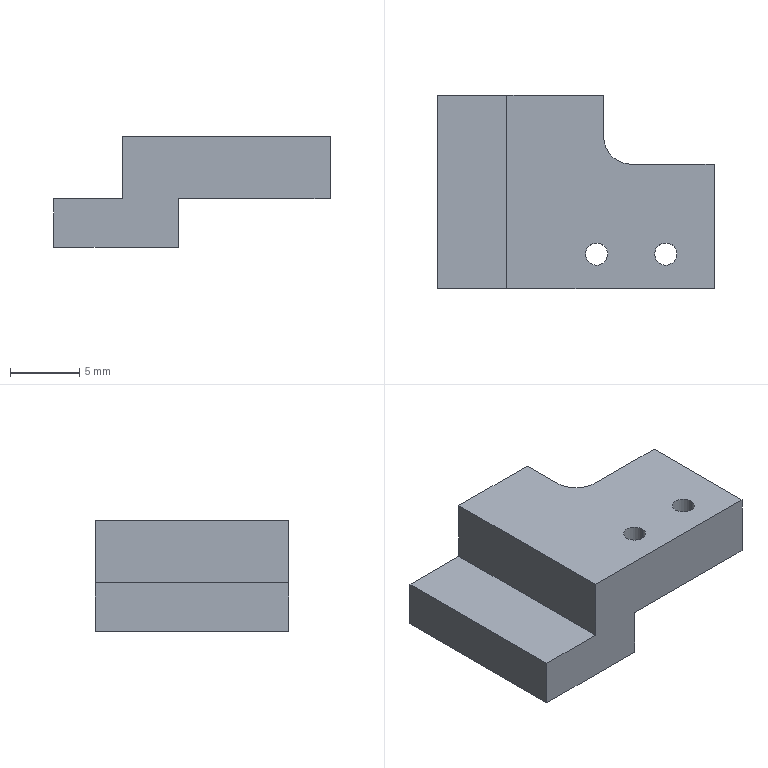Part | STEP file | FBDS-CS-024 | 1 solid | 19 faces | box 20 x 14 x 8 mm | volume 1034 mm3 | plane 14 | cylinder 5 | commonest cylinder face diameters 1.6 x4 4 x1
STEP:
#1=CARTESIAN_POINT('',(12.3,-11.5,5.));
#2=VERTEX_POINT('',#1);
#3=CARTESIAN_POINT('',(10.7,-11.5,5.));
#4=VERTEX_POINT('',#3);
#5=CARTESIAN_POINT('',(11.5,-11.5,5.));
#6=DIRECTION('',(0.,0.,-1.));
#7=DIRECTION('',(-1.,0.,0.));
#8=AXIS2_PLACEMENT_3D('',#5,#6,#7);
#9=CIRCLE('',#8,0.8);
#10=EDGE_CURVE('',#2,#4,#9,.T.);
#11=ORIENTED_EDGE('',*,*,#10,.T.);
#12=CARTESIAN_POINT('',(10.7,-11.5,8.));
#13=VERTEX_POINT('',#12);
#14=CARTESIAN_POINT('',(10.7,-11.5,8.));
#15=DIRECTION('',(0.,0.,1.));
#16=VECTOR('',#15,1000.);
#17=LINE('',#14,#16);
#18=EDGE_CURVE('',#4,#13,#17,.T.);
#19=ORIENTED_EDGE('',*,*,#18,.T.);
#20=CARTESIAN_POINT('',(12.3,-11.5,8.));
#21=VERTEX_POINT('',#20);
#22=CARTESIAN_POINT('',(11.5,-11.5,8.));
#23=DIRECTION('',(0.,0.,1.));
#24=DIRECTION('',(1.,0.,0.));
#25=AXIS2_PLACEMENT_3D('',#22,#23,#24);
#26=CIRCLE('',#25,0.8);
#27=EDGE_CURVE('',#13,#21,#26,.T.);
#28=ORIENTED_EDGE('',*,*,#27,.T.);
#29=CARTESIAN_POINT('',(12.3,-11.5,8.));
#30=DIRECTION('',(0.,0.,1.));
#31=VECTOR('',#30,1000.);
#32=LINE('',#29,#31);
#33=EDGE_CURVE('',#2,#21,#32,.T.);
#34=ORIENTED_EDGE('',*,*,#33,.F.);
#35=EDGE_LOOP('',(#11,#19,#28,#34));
#36=FACE_OUTER_BOUND('',#35,.T.);
#37=CARTESIAN_POINT('',(11.5,-11.5,8.));
#38=DIRECTION('',(0.,0.,1.));
#39=DIRECTION('',(1.,0.,0.));
#40=AXIS2_PLACEMENT_3D('',#37,#38,#39);
#41=CYLINDRICAL_SURFACE('',#40,0.8);
#42=ADVANCED_FACE('',(#36),#41,.F.);
#43=CARTESIAN_POINT('',(17.3,-11.5,5.));
#44=VERTEX_POINT('',#43);
#45=CARTESIAN_POINT('',(15.7,-11.5,5.));
#46=VERTEX_POINT('',#45);
#47=CARTESIAN_POINT('',(16.5,-11.5,5.));
#48=DIRECTION('',(0.,0.,-1.));
#49=DIRECTION('',(-1.,0.,0.));
#50=AXIS2_PLACEMENT_3D('',#47,#48,#49);
#51=CIRCLE('',#50,0.8);
#52=EDGE_CURVE('',#44,#46,#51,.T.);
#53=ORIENTED_EDGE('',*,*,#52,.T.);
#54=CARTESIAN_POINT('',(15.7,-11.5,8.));
#55=VERTEX_POINT('',#54);
#56=CARTESIAN_POINT('',(15.7,-11.5,8.));
#57=DIRECTION('',(0.,0.,1.));
#58=VECTOR('',#57,1000.);
#59=LINE('',#56,#58);
#60=EDGE_CURVE('',#46,#55,#59,.T.);
#61=ORIENTED_EDGE('',*,*,#60,.T.);
#62=CARTESIAN_POINT('',(17.3,-11.5,8.));
#63=VERTEX_POINT('',#62);
#64=CARTESIAN_POINT('',(16.5,-11.5,8.));
#65=DIRECTION('',(0.,0.,1.));
#66=DIRECTION('',(1.,0.,0.));
#67=AXIS2_PLACEMENT_3D('',#64,#65,#66);
#68=CIRCLE('',#67,0.8);
#69=EDGE_CURVE('',#55,#63,#68,.T.);
#70=ORIENTED_EDGE('',*,*,#69,.T.);
#71=CARTESIAN_POINT('',(17.3,-11.5,8.));
#72=DIRECTION('',(0.,0.,1.));
#73=VECTOR('',#72,1000.);
#74=LINE('',#71,#73);
#75=EDGE_CURVE('',#44,#63,#74,.T.);
#76=ORIENTED_EDGE('',*,*,#75,.F.);
#77=EDGE_LOOP('',(#53,#61,#70,#76));
#78=FACE_OUTER_BOUND('',#77,.T.);
#79=CARTESIAN_POINT('',(16.5,-11.5,8.));
#80=DIRECTION('',(0.,0.,1.));
#81=DIRECTION('',(1.,0.,0.));
#82=AXIS2_PLACEMENT_3D('',#79,#80,#81);
#83=CYLINDRICAL_SURFACE('',#82,0.8);
#84=ADVANCED_FACE('',(#78),#83,.F.);
#85=CARTESIAN_POINT('',(5.,-14.,3.5));
#86=VERTEX_POINT('',#85);
#87=CARTESIAN_POINT('',(0.,-14.,3.5));
#88=VERTEX_POINT('',#87);
#89=CARTESIAN_POINT('',(9.,-14.,3.5));
#90=DIRECTION('',(-1.,0.,0.));
#91=VECTOR('',#90,1000.);
#92=LINE('',#89,#91);
#93=EDGE_CURVE('',#86,#88,#92,.T.);
#94=ORIENTED_EDGE('',*,*,#93,.F.);
#95=CARTESIAN_POINT('',(5.,0.,3.5));
#96=VERTEX_POINT('',#95);
#97=CARTESIAN_POINT('',(5.,0.,3.5));
#98=DIRECTION('',(0.,1.,0.));
#99=VECTOR('',#98,1000.);
#100=LINE('',#97,#99);
#101=EDGE_CURVE('',#86,#96,#100,.T.);
#102=ORIENTED_EDGE('',*,*,#101,.T.);
#103=CARTESIAN_POINT('',(0.,0.,3.5));
#104=VERTEX_POINT('',#103);
#105=CARTESIAN_POINT('',(0.,0.,3.5));
#106=DIRECTION('',(-1.,0.,0.));
#107=VECTOR('',#106,1000.);
#108=LINE('',#105,#107);
#109=EDGE_CURVE('',#96,#104,#108,.T.);
#110=ORIENTED_EDGE('',*,*,#109,.T.);
#111=CARTESIAN_POINT('',(0.,0.,3.5));
#112=DIRECTION('',(0.,-1.,0.));
#113=VECTOR('',#112,1000.);
#114=LINE('',#111,#113);
#115=EDGE_CURVE('',#104,#88,#114,.T.);
#116=ORIENTED_EDGE('',*,*,#115,.T.);
#117=EDGE_LOOP('',(#94,#102,#110,#116));
#118=FACE_OUTER_BOUND('',#117,.T.);
#119=CARTESIAN_POINT('',(0.,0.,3.5));
#120=DIRECTION('',(0.,0.,1.));
#121=DIRECTION('',(1.,0.,0.));
#122=AXIS2_PLACEMENT_3D('',#119,#120,#121);
#123=PLANE('',#122);
#124=ADVANCED_FACE('',(#118),#123,.T.);
#125=CARTESIAN_POINT('',(9.,-14.,3.5));
#126=VERTEX_POINT('',#125);
#127=CARTESIAN_POINT('',(9.,-14.,0.));
#128=VERTEX_POINT('',#127);
#129=CARTESIAN_POINT('',(9.,-14.,8.64));
#130=DIRECTION('',(0.,0.,-1.));
#131=VECTOR('',#130,1000.);
#132=LINE('',#129,#131);
#133=EDGE_CURVE('',#126,#128,#132,.T.);
#134=ORIENTED_EDGE('',*,*,#133,.F.);
#135=CARTESIAN_POINT('',(20.,-14.,3.5));
#136=VERTEX_POINT('',#135);
#137=CARTESIAN_POINT('',(0.,-14.,3.5));
#138=DIRECTION('',(-1.,0.,0.));
#139=VECTOR('',#138,1000.);
#140=LINE('',#137,#139);
#141=EDGE_CURVE('',#136,#126,#140,.T.);
#142=ORIENTED_EDGE('',*,*,#141,.F.);
#143=CARTESIAN_POINT('',(20.,-14.,8.));
#144=VERTEX_POINT('',#143);
#145=CARTESIAN_POINT('',(20.,-14.,8.));
#146=DIRECTION('',(0.,0.,-1.));
#147=VECTOR('',#146,1000.);
#148=LINE('',#145,#147);
#149=EDGE_CURVE('',#144,#136,#148,.T.);
#150=ORIENTED_EDGE('',*,*,#149,.F.);
#151=CARTESIAN_POINT('',(5.,-14.,8.));
#152=VERTEX_POINT('',#151);
#153=CARTESIAN_POINT('',(0.,-14.,8.));
#154=DIRECTION('',(1.,0.,0.));
#155=VECTOR('',#154,1000.);
#156=LINE('',#153,#155);
#157=EDGE_CURVE('',#152,#144,#156,.T.);
#158=ORIENTED_EDGE('',*,*,#157,.F.);
#159=CARTESIAN_POINT('',(5.,-14.,-3.208));
#160=DIRECTION('',(0.,0.,1.));
#161=VECTOR('',#160,1000.);
#162=LINE('',#159,#161);
#163=EDGE_CURVE('',#86,#152,#162,.T.);
#164=ORIENTED_EDGE('',*,*,#163,.F.);
#165=ORIENTED_EDGE('',*,*,#93,.T.);
#166=CARTESIAN_POINT('',(0.,-14.,0.));
#167=VERTEX_POINT('',#166);
#168=CARTESIAN_POINT('',(0.,-14.,20.143));
#169=DIRECTION('',(0.,0.,-1.));
#170=VECTOR('',#169,1000.);
#171=LINE('',#168,#170);
#172=EDGE_CURVE('',#88,#167,#171,.T.);
#173=ORIENTED_EDGE('',*,*,#172,.T.);
#174=CARTESIAN_POINT('',(9.,-14.,0.));
#175=DIRECTION('',(-1.,0.,0.));
#176=VECTOR('',#175,1000.);
#177=LINE('',#174,#176);
#178=EDGE_CURVE('',#128,#167,#177,.T.);
#179=ORIENTED_EDGE('',*,*,#178,.F.);
#180=EDGE_LOOP('',(#134,#142,#150,#158,#164,#165,#173,#179));
#181=FACE_OUTER_BOUND('',#180,.T.);
#182=CARTESIAN_POINT('',(0.,-14.,8.));
#183=DIRECTION('',(0.,1.,0.));
#184=DIRECTION('',(0.,0.,1.));
#185=AXIS2_PLACEMENT_3D('',#182,#183,#184);
#186=PLANE('',#185);
#187=ADVANCED_FACE('',(#181),#186,.F.);
#188=CARTESIAN_POINT('',(20.,-13.5,3.5));
#189=VERTEX_POINT('',#188);
#190=CARTESIAN_POINT('',(20.,0.,3.5));
#191=DIRECTION('',(0.,-1.,0.));
#192=VECTOR('',#191,1000.);
#193=LINE('',#190,#192);
#194=EDGE_CURVE('',#189,#136,#193,.T.);
#195=ORIENTED_EDGE('',*,*,#194,.F.);
#196=CARTESIAN_POINT('',(20.,-13.5,5.));
#197=VERTEX_POINT('',#196);
#198=CARTESIAN_POINT('',(20.,-13.5,8.));
#199=DIRECTION('',(0.,0.,1.));
#200=VECTOR('',#199,1000.);
#201=LINE('',#198,#200);
#202=EDGE_CURVE('',#189,#197,#201,.T.);
#203=ORIENTED_EDGE('',*,*,#202,.T.);
#204=CARTESIAN_POINT('',(20.,-5.,5.));
#205=VERTEX_POINT('',#204);
#206=CARTESIAN_POINT('',(20.,0.,5.));
#207=DIRECTION('',(0.,-1.,0.));
#208=VECTOR('',#207,1000.);
#209=LINE('',#206,#208);
#210=EDGE_CURVE('',#205,#197,#209,.T.);
#211=ORIENTED_EDGE('',*,*,#210,.F.);
#212=CARTESIAN_POINT('',(20.,-5.,8.));
#213=VERTEX_POINT('',#212);
#214=CARTESIAN_POINT('',(20.,-5.,-2.5));
#215=DIRECTION('',(0.,0.,1.));
#216=VECTOR('',#215,1000.);
#217=LINE('',#214,#216);
#218=EDGE_CURVE('',#205,#213,#217,.T.);
#219=ORIENTED_EDGE('',*,*,#218,.T.);
#220=CARTESIAN_POINT('',(20.,0.,8.));
#221=DIRECTION('',(0.,1.,0.));
#222=VECTOR('',#221,1000.);
#223=LINE('',#220,#222);
#224=EDGE_CURVE('',#144,#213,#223,.T.);
#225=ORIENTED_EDGE('',*,*,#224,.F.);
#226=ORIENTED_EDGE('',*,*,#149,.T.);
#227=EDGE_LOOP('',(#195,#203,#211,#219,#225,#226));
#228=FACE_OUTER_BOUND('',#227,.T.);
#229=CARTESIAN_POINT('',(20.,0.,8.));
#230=DIRECTION('',(-1.,0.,0.));
#231=DIRECTION('',(0.,0.,1.));
#232=AXIS2_PLACEMENT_3D('',#229,#230,#231);
#233=PLANE('',#232);
#234=ADVANCED_FACE('',(#228),#233,.F.);
#235=CARTESIAN_POINT('',(9.,-13.5,3.5));
#236=VERTEX_POINT('',#235);
#237=CARTESIAN_POINT('',(28.367,-13.5,3.5));
#238=DIRECTION('',(1.,0.,0.));
#239=VECTOR('',#238,1000.);
#240=LINE('',#237,#239);
#241=EDGE_CURVE('',#236,#189,#240,.T.);
#242=ORIENTED_EDGE('',*,*,#241,.F.);
#243=CARTESIAN_POINT('',(9.,-13.5,5.));
#244=VERTEX_POINT('',#243);
#245=CARTESIAN_POINT('',(9.,-13.5,5.));
#246=DIRECTION('',(0.,0.,1.));
#247=VECTOR('',#246,1000.);
#248=LINE('',#245,#247);
#249=EDGE_CURVE('',#236,#244,#248,.T.);
#250=ORIENTED_EDGE('',*,*,#249,.T.);
#251=CARTESIAN_POINT('',(28.367,-13.5,5.));
#252=DIRECTION('',(-1.,0.,0.));
#253=VECTOR('',#252,1000.);
#254=LINE('',#251,#253);
#255=EDGE_CURVE('',#197,#244,#254,.T.);
#256=ORIENTED_EDGE('',*,*,#255,.F.);
#257=ORIENTED_EDGE('',*,*,#202,.F.);
#258=EDGE_LOOP('',(#242,#250,#256,#257));
#259=FACE_OUTER_BOUND('',#258,.T.);
#260=CARTESIAN_POINT('',(28.367,-13.5,5.));
#261=DIRECTION('',(0.,-1.,0.));
#262=DIRECTION('',(0.,0.,-1.));
#263=AXIS2_PLACEMENT_3D('',#260,#261,#262);
#264=PLANE('',#263);
#265=ADVANCED_FACE('',(#259),#264,.F.);
#266=CARTESIAN_POINT('',(9.,0.,0.));
#267=VERTEX_POINT('',#266);
#268=CARTESIAN_POINT('',(9.,1.393,0.));
#269=DIRECTION('',(0.,1.,0.));
#270=VECTOR('',#269,1000.);
#271=LINE('',#268,#270);
#272=EDGE_CURVE('',#128,#267,#271,.T.);
#273=ORIENTED_EDGE('',*,*,#272,.F.);
#274=ORIENTED_EDGE('',*,*,#178,.T.);
#275=CARTESIAN_POINT('',(0.,0.,0.));
#276=VERTEX_POINT('',#275);
#277=CARTESIAN_POINT('',(0.,0.,0.));
#278=DIRECTION('',(0.,-1.,0.));
#279=VECTOR('',#278,1000.);
#280=LINE('',#277,#279);
#281=EDGE_CURVE('',#276,#167,#280,.T.);
#282=ORIENTED_EDGE('',*,*,#281,.F.);
#283=CARTESIAN_POINT('',(0.,0.,0.));
#284=DIRECTION('',(-1.,0.,0.));
#285=VECTOR('',#284,1000.);
#286=LINE('',#283,#285);
#287=EDGE_CURVE('',#267,#276,#286,.T.);
#288=ORIENTED_EDGE('',*,*,#287,.F.);
#289=EDGE_LOOP('',(#273,#274,#282,#288));
#290=FACE_OUTER_BOUND('',#289,.T.);
#291=CARTESIAN_POINT('',(0.,0.,0.));
#292=DIRECTION('',(0.,0.,1.));
#293=DIRECTION('',(1.,0.,0.));
#294=AXIS2_PLACEMENT_3D('',#291,#292,#293);
#295=PLANE('',#294);
#296=ADVANCED_FACE('',(#290),#295,.F.);
#297=CARTESIAN_POINT('',(9.,0.,5.));
#298=VERTEX_POINT('',#297);
#299=CARTESIAN_POINT('',(9.,1.393,5.));
#300=DIRECTION('',(0.,1.,0.));
#301=VECTOR('',#300,1000.);
#302=LINE('',#299,#301);
#303=EDGE_CURVE('',#244,#298,#302,.T.);
#304=ORIENTED_EDGE('',*,*,#303,.F.);
#305=ORIENTED_EDGE('',*,*,#249,.F.);
#306=CARTESIAN_POINT('',(9.,0.,3.5));
#307=DIRECTION('',(0.,-1.,0.));
#308=VECTOR('',#307,1000.);
#309=LINE('',#306,#308);
#310=EDGE_CURVE('',#236,#126,#309,.T.);
#311=ORIENTED_EDGE('',*,*,#310,.T.);
#312=ORIENTED_EDGE('',*,*,#133,.T.);
#313=ORIENTED_EDGE('',*,*,#272,.T.);
#314=CARTESIAN_POINT('',(9.,0.,8.));
#315=DIRECTION('',(0.,0.,-1.));
#316=VECTOR('',#315,1000.);
#317=LINE('',#314,#316);
#318=EDGE_CURVE('',#298,#267,#317,.T.);
#319=ORIENTED_EDGE('',*,*,#318,.F.);
#320=EDGE_LOOP('',(#304,#305,#311,#312,#313,#319));
#321=FACE_OUTER_BOUND('',#320,.T.);
#322=CARTESIAN_POINT('',(9.,1.393,5.));
#323=DIRECTION('',(-1.,0.,0.));
#324=DIRECTION('',(0.,-1.,0.));
#325=AXIS2_PLACEMENT_3D('',#322,#323,#324);
#326=PLANE('',#325);
#327=ADVANCED_FACE('',(#321),#326,.F.);
#328=CARTESIAN_POINT('',(14.,-5.,5.));
#329=VERTEX_POINT('',#328);
#330=CARTESIAN_POINT('',(20.,-5.,5.));
#331=DIRECTION('',(1.,0.,0.));
#332=VECTOR('',#331,1000.);
#333=LINE('',#330,#332);
#334=EDGE_CURVE('',#329,#205,#333,.T.);
#335=ORIENTED_EDGE('',*,*,#334,.F.);
#336=CARTESIAN_POINT('',(14.,-5.,8.));
#337=VERTEX_POINT('',#336);
#338=CARTESIAN_POINT('',(14.,-5.,8.));
#339=DIRECTION('',(0.,0.,1.));
#340=VECTOR('',#339,1000.);
#341=LINE('',#338,#340);
#342=EDGE_CURVE('',#329,#337,#341,.T.);
#343=ORIENTED_EDGE('',*,*,#342,.T.);
#344=CARTESIAN_POINT('',(20.,-5.,8.));
#345=DIRECTION('',(1.,0.,0.));
#346=VECTOR('',#345,1000.);
#347=LINE('',#344,#346);
#348=EDGE_CURVE('',#337,#213,#347,.T.);
#349=ORIENTED_EDGE('',*,*,#348,.T.);
#350=ORIENTED_EDGE('',*,*,#218,.F.);
#351=EDGE_LOOP('',(#335,#343,#349,#350));
#352=FACE_OUTER_BOUND('',#351,.T.);
#353=CARTESIAN_POINT('',(20.,-5.,-2.5));
#354=DIRECTION('',(0.,-1.,0.));
#355=DIRECTION('',(1.,0.,0.));
#356=AXIS2_PLACEMENT_3D('',#353,#354,#355);
#357=PLANE('',#356);
#358=ADVANCED_FACE('',(#352),#357,.F.);
#359=CARTESIAN_POINT('',(12.,0.,8.));
#360=VERTEX_POINT('',#359);
#361=CARTESIAN_POINT('',(12.,-3.,8.));
#362=VERTEX_POINT('',#361);
#363=CARTESIAN_POINT('',(12.,0.,8.));
#364=DIRECTION('',(0.,-1.,0.));
#365=VECTOR('',#364,1000.);
#366=LINE('',#363,#365);
#367=EDGE_CURVE('',#360,#362,#366,.T.);
#368=ORIENTED_EDGE('',*,*,#367,.T.);
#369=CARTESIAN_POINT('',(12.,-3.,5.));
#370=VERTEX_POINT('',#369);
#371=CARTESIAN_POINT('',(12.,-3.,5.));
#372=DIRECTION('',(0.,0.,-1.));
#373=VECTOR('',#372,1000.);
#374=LINE('',#371,#373);
#375=EDGE_CURVE('',#362,#370,#374,.T.);
#376=ORIENTED_EDGE('',*,*,#375,.T.);
#377=CARTESIAN_POINT('',(12.,0.,5.));
#378=VERTEX_POINT('',#377);
#379=CARTESIAN_POINT('',(12.,0.,5.));
#380=DIRECTION('',(0.,-1.,0.));
#381=VECTOR('',#380,1000.);
#382=LINE('',#379,#381);
#383=EDGE_CURVE('',#378,#370,#382,.T.);
#384=ORIENTED_EDGE('',*,*,#383,.F.);
#385=CARTESIAN_POINT('',(12.,0.,-2.5));
#386=DIRECTION('',(0.,0.,1.));
#387=VECTOR('',#386,1000.);
#388=LINE('',#385,#387);
#389=EDGE_CURVE('',#378,#360,#388,.T.);
#390=ORIENTED_EDGE('',*,*,#389,.T.);
#391=EDGE_LOOP('',(#368,#376,#384,#390));
#392=FACE_OUTER_BOUND('',#391,.T.);
#393=CARTESIAN_POINT('',(12.,0.,-2.5));
#394=DIRECTION('',(-1.,0.,0.));
#395=DIRECTION('',(0.,0.,1.));
#396=AXIS2_PLACEMENT_3D('',#393,#394,#395);
#397=PLANE('',#396);
#398=ADVANCED_FACE('',(#392),#397,.F.);
#399=ORIENTED_EDGE('',*,*,#115,.F.);
#400=CARTESIAN_POINT('',(0.,0.,8.));
#401=DIRECTION('',(0.,0.,-1.));
#402=VECTOR('',#401,1000.);
#403=LINE('',#400,#402);
#404=EDGE_CURVE('',#104,#276,#403,.T.);
#405=ORIENTED_EDGE('',*,*,#404,.T.);
#406=ORIENTED_EDGE('',*,*,#281,.T.);
#407=ORIENTED_EDGE('',*,*,#172,.F.);
#408=EDGE_LOOP('',(#399,#405,#406,#407));
#409=FACE_OUTER_BOUND('',#408,.T.);
#410=CARTESIAN_POINT('',(0.,0.,8.));
#411=DIRECTION('',(1.,0.,0.));
#412=DIRECTION('',(0.,1.,0.));
#413=AXIS2_PLACEMENT_3D('',#410,#411,#412);
#414=PLANE('',#413);
#415=ADVANCED_FACE('',(#409),#414,.F.);
#416=ORIENTED_EDGE('',*,*,#318,.T.);
#417=ORIENTED_EDGE('',*,*,#287,.T.);
#418=ORIENTED_EDGE('',*,*,#404,.F.);
#419=ORIENTED_EDGE('',*,*,#109,.F.);
#420=CARTESIAN_POINT('',(5.,0.,8.));
#421=VERTEX_POINT('',#420);
#422=CARTESIAN_POINT('',(5.,0.,3.5));
#423=DIRECTION('',(0.,0.,1.));
#424=VECTOR('',#423,1000.);
#425=LINE('',#422,#424);
#426=EDGE_CURVE('',#96,#421,#425,.T.);
#427=ORIENTED_EDGE('',*,*,#426,.T.);
#428=CARTESIAN_POINT('',(0.,0.,8.));
#429=DIRECTION('',(-1.,0.,0.));
#430=VECTOR('',#429,1000.);
#431=LINE('',#428,#430);
#432=EDGE_CURVE('',#360,#421,#431,.T.);
#433=ORIENTED_EDGE('',*,*,#432,.F.);
#434=ORIENTED_EDGE('',*,*,#389,.F.);
#435=CARTESIAN_POINT('',(0.,0.,5.));
#436=DIRECTION('',(1.,0.,0.));
#437=VECTOR('',#436,1000.);
#438=LINE('',#435,#437);
#439=EDGE_CURVE('',#298,#378,#438,.T.);
#440=ORIENTED_EDGE('',*,*,#439,.F.);
#441=EDGE_LOOP('',(#416,#417,#418,#419,#427,#433,#434,#440));
#442=FACE_OUTER_BOUND('',#441,.T.);
#443=CARTESIAN_POINT('',(0.,0.,8.));
#444=DIRECTION('',(0.,-1.,0.));
#445=DIRECTION('',(0.,0.,-1.));
#446=AXIS2_PLACEMENT_3D('',#443,#444,#445);
#447=PLANE('',#446);
#448=ADVANCED_FACE('',(#442),#447,.F.);
#449=CARTESIAN_POINT('',(5.,0.,8.));
#450=DIRECTION('',(0.,1.,0.));
#451=VECTOR('',#450,1000.);
#452=LINE('',#449,#451);
#453=EDGE_CURVE('',#152,#421,#452,.T.);
#454=ORIENTED_EDGE('',*,*,#453,.F.);
#455=ORIENTED_EDGE('',*,*,#157,.T.);
#456=ORIENTED_EDGE('',*,*,#224,.T.);
#457=ORIENTED_EDGE('',*,*,#348,.F.);
#458=CARTESIAN_POINT('',(14.,-3.,8.));
#459=DIRECTION('',(0.,0.,-1.));
#460=DIRECTION('',(1.,0.,0.));
#461=AXIS2_PLACEMENT_3D('',#458,#459,#460);
#462=CIRCLE('',#461,2.);
#463=EDGE_CURVE('',#337,#362,#462,.T.);
#464=ORIENTED_EDGE('',*,*,#463,.T.);
#465=ORIENTED_EDGE('',*,*,#367,.F.);
#466=ORIENTED_EDGE('',*,*,#432,.T.);
#467=EDGE_LOOP('',(#454,#455,#456,#457,#464,#465,#466));
#468=FACE_OUTER_BOUND('',#467,.T.);
#469=CARTESIAN_POINT('',(11.5,-11.5,8.));
#470=DIRECTION('',(0.,0.,1.));
#471=DIRECTION('',(1.,0.,0.));
#472=AXIS2_PLACEMENT_3D('',#469,#470,#471);
#473=CIRCLE('',#472,0.8);
#474=EDGE_CURVE('',#21,#13,#473,.T.);
#475=ORIENTED_EDGE('',*,*,#474,.F.);
#476=ORIENTED_EDGE('',*,*,#27,.F.);
#477=EDGE_LOOP('',(#475,#476));
#478=FACE_BOUND('',#477,.T.);
#479=CARTESIAN_POINT('',(16.5,-11.5,8.));
#480=DIRECTION('',(0.,0.,1.));
#481=DIRECTION('',(1.,0.,0.));
#482=AXIS2_PLACEMENT_3D('',#479,#480,#481);
#483=CIRCLE('',#482,0.8);
#484=EDGE_CURVE('',#63,#55,#483,.T.);
#485=ORIENTED_EDGE('',*,*,#484,.F.);
#486=ORIENTED_EDGE('',*,*,#69,.F.);
#487=EDGE_LOOP('',(#485,#486));
#488=FACE_BOUND('',#487,.T.);
#489=CARTESIAN_POINT('',(0.,0.,8.));
#490=DIRECTION('',(0.,0.,1.));
#491=DIRECTION('',(1.,0.,0.));
#492=AXIS2_PLACEMENT_3D('',#489,#490,#491);
#493=PLANE('',#492);
#494=ADVANCED_FACE('',(#468,#478,#488),#493,.T.);
#495=ORIENTED_EDGE('',*,*,#453,.T.);
#496=ORIENTED_EDGE('',*,*,#426,.F.);
#497=ORIENTED_EDGE('',*,*,#101,.F.);
#498=ORIENTED_EDGE('',*,*,#163,.T.);
#499=EDGE_LOOP('',(#495,#496,#497,#498));
#500=FACE_OUTER_BOUND('',#499,.T.);
#501=CARTESIAN_POINT('',(5.,0.,3.5));
#502=DIRECTION('',(1.,0.,0.));
#503=DIRECTION('',(0.,1.,0.));
#504=AXIS2_PLACEMENT_3D('',#501,#502,#503);
#505=PLANE('',#504);
#506=ADVANCED_FACE('',(#500),#505,.F.);
#507=ORIENTED_EDGE('',*,*,#255,.T.);
#508=ORIENTED_EDGE('',*,*,#303,.T.);
#509=ORIENTED_EDGE('',*,*,#439,.T.);
#510=ORIENTED_EDGE('',*,*,#383,.T.);
#511=CARTESIAN_POINT('',(14.,-3.,5.));
#512=DIRECTION('',(0.,0.,1.));
#513=DIRECTION('',(-1.,0.,0.));
#514=AXIS2_PLACEMENT_3D('',#511,#512,#513);
#515=CIRCLE('',#514,2.);
#516=EDGE_CURVE('',#370,#329,#515,.T.);
#517=ORIENTED_EDGE('',*,*,#516,.T.);
#518=ORIENTED_EDGE('',*,*,#334,.T.);
#519=ORIENTED_EDGE('',*,*,#210,.T.);
#520=EDGE_LOOP('',(#507,#508,#509,#510,#517,#518,#519));
#521=FACE_OUTER_BOUND('',#520,.T.);
#522=ORIENTED_EDGE('',*,*,#10,.F.);
#523=CARTESIAN_POINT('',(11.5,-11.5,5.));
#524=DIRECTION('',(0.,0.,-1.));
#525=DIRECTION('',(-1.,0.,0.));
#526=AXIS2_PLACEMENT_3D('',#523,#524,#525);
#527=CIRCLE('',#526,0.8);
#528=EDGE_CURVE('',#4,#2,#527,.T.);
#529=ORIENTED_EDGE('',*,*,#528,.F.);
#530=EDGE_LOOP('',(#522,#529));
#531=FACE_BOUND('',#530,.T.);
#532=ORIENTED_EDGE('',*,*,#52,.F.);
#533=CARTESIAN_POINT('',(16.5,-11.5,5.));
#534=DIRECTION('',(0.,0.,-1.));
#535=DIRECTION('',(-1.,0.,0.));
#536=AXIS2_PLACEMENT_3D('',#533,#534,#535);
#537=CIRCLE('',#536,0.8);
#538=EDGE_CURVE('',#46,#44,#537,.T.);
#539=ORIENTED_EDGE('',*,*,#538,.F.);
#540=EDGE_LOOP('',(#532,#539));
#541=FACE_BOUND('',#540,.T.);
#542=CARTESIAN_POINT('',(0.,0.,5.));
#543=DIRECTION('',(0.,0.,-1.));
#544=DIRECTION('',(-1.,0.,0.));
#545=AXIS2_PLACEMENT_3D('',#542,#543,#544);
#546=PLANE('',#545);
#547=ADVANCED_FACE('',(#521,#531,#541),#546,.T.);
#548=ORIENTED_EDGE('',*,*,#60,.F.);
#549=ORIENTED_EDGE('',*,*,#538,.T.);
#550=ORIENTED_EDGE('',*,*,#75,.T.);
#551=ORIENTED_EDGE('',*,*,#484,.T.);
#552=EDGE_LOOP('',(#548,#549,#550,#551));
#553=FACE_OUTER_BOUND('',#552,.T.);
#554=CARTESIAN_POINT('',(16.5,-11.5,8.));
#555=DIRECTION('',(0.,0.,1.));
#556=DIRECTION('',(1.,0.,0.));
#557=AXIS2_PLACEMENT_3D('',#554,#555,#556);
#558=CYLINDRICAL_SURFACE('',#557,0.8);
#559=ADVANCED_FACE('',(#553),#558,.F.);
#560=ORIENTED_EDGE('',*,*,#18,.F.);
#561=ORIENTED_EDGE('',*,*,#528,.T.);
#562=ORIENTED_EDGE('',*,*,#33,.T.);
#563=ORIENTED_EDGE('',*,*,#474,.T.);
#564=EDGE_LOOP('',(#560,#561,#562,#563));
#565=FACE_OUTER_BOUND('',#564,.T.);
#566=CARTESIAN_POINT('',(11.5,-11.5,8.));
#567=DIRECTION('',(0.,0.,1.));
#568=DIRECTION('',(1.,0.,0.));
#569=AXIS2_PLACEMENT_3D('',#566,#567,#568);
#570=CYLINDRICAL_SURFACE('',#569,0.8);
#571=ADVANCED_FACE('',(#565),#570,.F.);
#572=ORIENTED_EDGE('',*,*,#516,.F.);
#573=ORIENTED_EDGE('',*,*,#375,.F.);
#574=ORIENTED_EDGE('',*,*,#463,.F.);
#575=ORIENTED_EDGE('',*,*,#342,.F.);
#576=EDGE_LOOP('',(#572,#573,#574,#575));
#577=FACE_OUTER_BOUND('',#576,.T.);
#578=CARTESIAN_POINT('',(14.,-3.,-2.5));
#579=DIRECTION('',(0.,0.,-1.));
#580=DIRECTION('',(-1.,0.,0.));
#581=AXIS2_PLACEMENT_3D('',#578,#579,#580);
#582=CYLINDRICAL_SURFACE('',#581,2.);
#583=ADVANCED_FACE('',(#577),#582,.F.);
#584=ORIENTED_EDGE('',*,*,#310,.F.);
#585=ORIENTED_EDGE('',*,*,#241,.T.);
#586=ORIENTED_EDGE('',*,*,#194,.T.);
#587=ORIENTED_EDGE('',*,*,#141,.T.);
#588=EDGE_LOOP('',(#584,#585,#586,#587));
#589=FACE_OUTER_BOUND('',#588,.T.);
#590=CARTESIAN_POINT('',(0.,0.,3.5));
#591=DIRECTION('',(0.,0.,-1.));
#592=DIRECTION('',(-1.,0.,0.));
#593=AXIS2_PLACEMENT_3D('',#590,#591,#592);
#594=PLANE('',#593);
#595=ADVANCED_FACE('',(#589),#594,.T.);
#596=CLOSED_SHELL('',(#42,#84,#124,#187,#234,#265,#296,#327,#358,#398,#415,#448,#494,#506,#547,#559,#571,#583,#595));
#597=MANIFOLD_SOLID_BREP('',#596);
#598=CARTESIAN_POINT('',(0.,0.,0.));
#599=DIRECTION('',(0.,0.,1.));
#600=DIRECTION('',(1.,0.,0.));
#601=AXIS2_PLACEMENT_3D('',#598,#599,#600);
#602=(LENGTH_UNIT()NAMED_UNIT(*)SI_UNIT(.MILLI.,.METRE.));
#603=UNCERTAINTY_MEASURE_WITH_UNIT(LENGTH_MEASURE(0.00001),#602,'','');
#604=(NAMED_UNIT(*)PLANE_ANGLE_UNIT()SI_UNIT($,.RADIAN.));
#605=(NAMED_UNIT(*)SI_UNIT($,.STERADIAN.)SOLID_ANGLE_UNIT());
#606=(GEOMETRIC_REPRESENTATION_CONTEXT(3)GLOBAL_UNCERTAINTY_ASSIGNED_CONTEXT((#603))GLOBAL_UNIT_ASSIGNED_CONTEXT((#602,#604,#605))REPRESENTATION_CONTEXT('',''));
#607=ADVANCED_BREP_SHAPE_REPRESENTATION('',(#597,#601),#606);